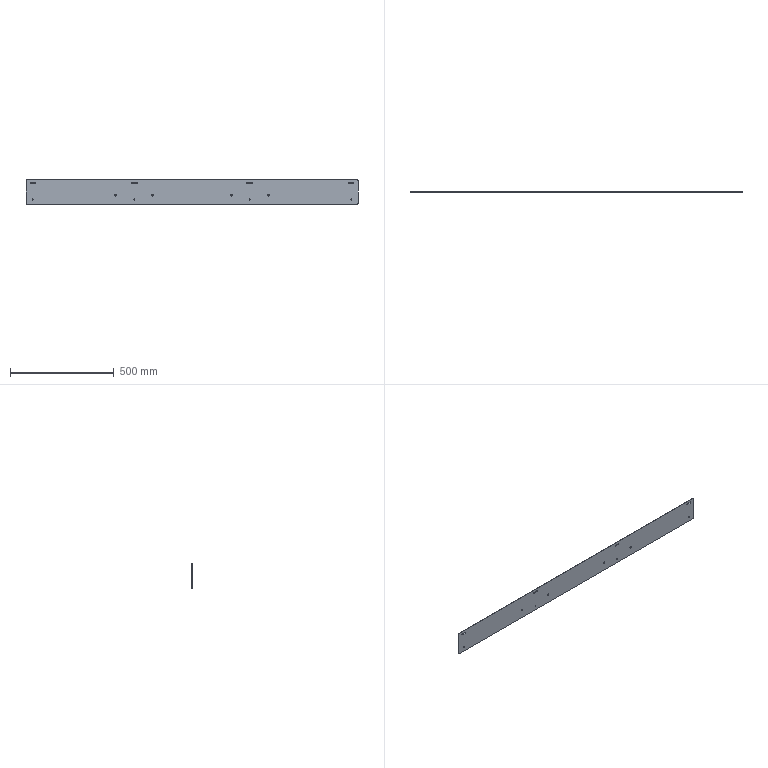Part | NX | features BREP 1 | 1 solid | 42 faces | box 1600 x 3 x 120 mm | volume 573268 mm3 | cylinder 28 | plane 14 | commonest cylinder face diameters 5.5 x8 6 x8 8 x8 10 x4
STEP:
#1=CARTESIAN_POINT('',(-800.,0.,-55.));
#2=VERTEX_POINT('',#1);
#3=CARTESIAN_POINT('',(-800.,0.,55.));
#4=VERTEX_POINT('',#3);
#5=CARTESIAN_POINT('',(-800.,0.,-55.));
#6=DIRECTION('',(0.,0.,1.));
#7=VECTOR('',#6,1000.);
#8=LINE('',#5,#7);
#9=EDGE_CURVE('',#2,#4,#8,.T.);
#10=ORIENTED_EDGE('',*,*,#9,.T.);
#11=CARTESIAN_POINT('',(-795.,0.,60.));
#12=VERTEX_POINT('',#11);
#13=CARTESIAN_POINT('',(-795.,0.,55.));
#14=DIRECTION('',(0.,1.,0.));
#15=DIRECTION('',(-1.,0.,0.));
#16=AXIS2_PLACEMENT_3D('',#13,#14,#15);
#17=CIRCLE('',#16,5.);
#18=EDGE_CURVE('',#4,#12,#17,.T.);
#19=ORIENTED_EDGE('',*,*,#18,.T.);
#20=CARTESIAN_POINT('',(795.,0.,60.));
#21=VERTEX_POINT('',#20);
#22=CARTESIAN_POINT('',(-795.,0.,60.));
#23=DIRECTION('',(1.,0.,0.));
#24=VECTOR('',#23,1000.);
#25=LINE('',#22,#24);
#26=EDGE_CURVE('',#12,#21,#25,.T.);
#27=ORIENTED_EDGE('',*,*,#26,.T.);
#28=CARTESIAN_POINT('',(800.,0.,55.));
#29=VERTEX_POINT('',#28);
#30=CARTESIAN_POINT('',(795.,0.,55.));
#31=DIRECTION('',(0.,1.,0.));
#32=DIRECTION('',(0.,0.,1.));
#33=AXIS2_PLACEMENT_3D('',#30,#31,#32);
#34=CIRCLE('',#33,5.);
#35=EDGE_CURVE('',#21,#29,#34,.T.);
#36=ORIENTED_EDGE('',*,*,#35,.T.);
#37=CARTESIAN_POINT('',(800.,0.,-55.));
#38=VERTEX_POINT('',#37);
#39=CARTESIAN_POINT('',(800.,0.,55.));
#40=DIRECTION('',(0.,0.,-1.));
#41=VECTOR('',#40,1000.);
#42=LINE('',#39,#41);
#43=EDGE_CURVE('',#29,#38,#42,.T.);
#44=ORIENTED_EDGE('',*,*,#43,.T.);
#45=CARTESIAN_POINT('',(795.,0.,-60.));
#46=VERTEX_POINT('',#45);
#47=CARTESIAN_POINT('',(795.,0.,-55.));
#48=DIRECTION('',(0.,1.,0.));
#49=DIRECTION('',(1.,0.,0.));
#50=AXIS2_PLACEMENT_3D('',#47,#48,#49);
#51=CIRCLE('',#50,5.);
#52=EDGE_CURVE('',#38,#46,#51,.T.);
#53=ORIENTED_EDGE('',*,*,#52,.T.);
#54=CARTESIAN_POINT('',(-795.,0.,-60.));
#55=VERTEX_POINT('',#54);
#56=CARTESIAN_POINT('',(795.,0.,-60.));
#57=DIRECTION('',(-1.,0.,0.));
#58=VECTOR('',#57,1000.);
#59=LINE('',#56,#58);
#60=EDGE_CURVE('',#46,#55,#59,.T.);
#61=ORIENTED_EDGE('',*,*,#60,.T.);
#62=CARTESIAN_POINT('',(-795.,0.,-55.));
#63=DIRECTION('',(0.,1.,0.));
#64=DIRECTION('',(0.,0.,-1.));
#65=AXIS2_PLACEMENT_3D('',#62,#63,#64);
#66=CIRCLE('',#65,5.);
#67=EDGE_CURVE('',#55,#2,#66,.T.);
#68=ORIENTED_EDGE('',*,*,#67,.T.);
#69=EDGE_LOOP('',(#10,#19,#27,#36,#44,#53,#61,#68));
#70=FACE_BOUND('',#69,.T.);
#71=CARTESIAN_POINT('',(-366.,0.,-15.34));
#72=VERTEX_POINT('',#71);
#73=CARTESIAN_POINT('',(-374.,0.,-15.34));
#74=VERTEX_POINT('',#73);
#75=CARTESIAN_POINT('',(-370.,0.,-15.34));
#76=DIRECTION('',(0.,1.,0.));
#77=DIRECTION('',(1.,0.,0.));
#78=AXIS2_PLACEMENT_3D('',#75,#76,#77);
#79=CIRCLE('',#78,4.);
#80=EDGE_CURVE('',#72,#74,#79,.T.);
#81=ORIENTED_EDGE('',*,*,#80,.F.);
#82=CARTESIAN_POINT('',(-370.,0.,-15.34));
#83=DIRECTION('',(0.,1.,0.));
#84=DIRECTION('',(-1.,0.,0.));
#85=AXIS2_PLACEMENT_3D('',#82,#83,#84);
#86=CIRCLE('',#85,4.);
#87=EDGE_CURVE('',#74,#72,#86,.T.);
#88=ORIENTED_EDGE('',*,*,#87,.F.);
#89=EDGE_LOOP('',(#81,#88));
#90=FACE_BOUND('',#89,.T.);
#91=CARTESIAN_POINT('',(-186.,0.,-15.34));
#92=VERTEX_POINT('',#91);
#93=CARTESIAN_POINT('',(-194.,0.,-15.34));
#94=VERTEX_POINT('',#93);
#95=CARTESIAN_POINT('',(-190.,0.,-15.34));
#96=DIRECTION('',(0.,1.,0.));
#97=DIRECTION('',(1.,0.,0.));
#98=AXIS2_PLACEMENT_3D('',#95,#96,#97);
#99=CIRCLE('',#98,4.);
#100=EDGE_CURVE('',#92,#94,#99,.T.);
#101=ORIENTED_EDGE('',*,*,#100,.F.);
#102=CARTESIAN_POINT('',(-190.,0.,-15.34));
#103=DIRECTION('',(0.,1.,0.));
#104=DIRECTION('',(-1.,0.,0.));
#105=AXIS2_PLACEMENT_3D('',#102,#103,#104);
#106=CIRCLE('',#105,4.);
#107=EDGE_CURVE('',#94,#92,#106,.T.);
#108=ORIENTED_EDGE('',*,*,#107,.F.);
#109=EDGE_LOOP('',(#101,#108));
#110=FACE_BOUND('',#109,.T.);
#111=CARTESIAN_POINT('',(194.,0.,-15.34));
#112=VERTEX_POINT('',#111);
#113=CARTESIAN_POINT('',(186.,0.,-15.34));
#114=VERTEX_POINT('',#113);
#115=CARTESIAN_POINT('',(190.,0.,-15.34));
#116=DIRECTION('',(0.,1.,0.));
#117=DIRECTION('',(1.,0.,0.));
#118=AXIS2_PLACEMENT_3D('',#115,#116,#117);
#119=CIRCLE('',#118,4.);
#120=EDGE_CURVE('',#112,#114,#119,.T.);
#121=ORIENTED_EDGE('',*,*,#120,.F.);
#122=CARTESIAN_POINT('',(190.,0.,-15.34));
#123=DIRECTION('',(0.,1.,0.));
#124=DIRECTION('',(-1.,0.,0.));
#125=AXIS2_PLACEMENT_3D('',#122,#123,#124);
#126=CIRCLE('',#125,4.);
#127=EDGE_CURVE('',#114,#112,#126,.T.);
#128=ORIENTED_EDGE('',*,*,#127,.F.);
#129=EDGE_LOOP('',(#121,#128));
#130=FACE_BOUND('',#129,.T.);
#131=CARTESIAN_POINT('',(374.,0.,-15.34));
#132=VERTEX_POINT('',#131);
#133=CARTESIAN_POINT('',(366.,0.,-15.34));
#134=VERTEX_POINT('',#133);
#135=CARTESIAN_POINT('',(370.,0.,-15.34));
#136=DIRECTION('',(0.,1.,0.));
#137=DIRECTION('',(1.,0.,0.));
#138=AXIS2_PLACEMENT_3D('',#135,#136,#137);
#139=CIRCLE('',#138,4.);
#140=EDGE_CURVE('',#132,#134,#139,.T.);
#141=ORIENTED_EDGE('',*,*,#140,.F.);
#142=CARTESIAN_POINT('',(370.,0.,-15.34));
#143=DIRECTION('',(0.,1.,0.));
#144=DIRECTION('',(-1.,0.,0.));
#145=AXIS2_PLACEMENT_3D('',#142,#143,#144);
#146=CIRCLE('',#145,4.);
#147=EDGE_CURVE('',#134,#132,#146,.T.);
#148=ORIENTED_EDGE('',*,*,#147,.F.);
#149=EDGE_LOOP('',(#141,#148));
#150=FACE_BOUND('',#149,.T.);
#151=CARTESIAN_POINT('',(757.5,0.,48.));
#152=VERTEX_POINT('',#151);
#153=CARTESIAN_POINT('',(777.5,0.,48.));
#154=VERTEX_POINT('',#153);
#155=CARTESIAN_POINT('',(757.5,0.,48.));
#156=DIRECTION('',(1.,0.,0.));
#157=VECTOR('',#156,1000.);
#158=LINE('',#155,#157);
#159=EDGE_CURVE('',#152,#154,#158,.T.);
#160=ORIENTED_EDGE('',*,*,#159,.F.);
#161=CARTESIAN_POINT('',(757.5,0.,42.));
#162=VERTEX_POINT('',#161);
#163=CARTESIAN_POINT('',(757.5,0.,45.));
#164=DIRECTION('',(0.,-1.,0.));
#165=DIRECTION('',(0.,0.,1.));
#166=AXIS2_PLACEMENT_3D('',#163,#164,#165);
#167=CIRCLE('',#166,3.);
#168=EDGE_CURVE('',#152,#162,#167,.T.);
#169=ORIENTED_EDGE('',*,*,#168,.T.);
#170=CARTESIAN_POINT('',(777.5,0.,42.));
#171=VERTEX_POINT('',#170);
#172=CARTESIAN_POINT('',(777.5,0.,42.));
#173=DIRECTION('',(-1.,0.,0.));
#174=VECTOR('',#173,1000.);
#175=LINE('',#172,#174);
#176=EDGE_CURVE('',#171,#162,#175,.T.);
#177=ORIENTED_EDGE('',*,*,#176,.F.);
#178=CARTESIAN_POINT('',(777.5,0.,45.));
#179=DIRECTION('',(0.,-1.,0.));
#180=DIRECTION('',(0.,0.,-1.));
#181=AXIS2_PLACEMENT_3D('',#178,#179,#180);
#182=CIRCLE('',#181,3.);
#183=EDGE_CURVE('',#171,#154,#182,.T.);
#184=ORIENTED_EDGE('',*,*,#183,.T.);
#185=EDGE_LOOP('',(#160,#169,#177,#184));
#186=FACE_BOUND('',#185,.T.);
#187=CARTESIAN_POINT('',(287.5,0.,42.));
#188=VERTEX_POINT('',#187);
#189=CARTESIAN_POINT('',(267.5,0.,42.));
#190=VERTEX_POINT('',#189);
#191=CARTESIAN_POINT('',(287.5,0.,42.));
#192=DIRECTION('',(-1.,0.,0.));
#193=VECTOR('',#192,1000.);
#194=LINE('',#191,#193);
#195=EDGE_CURVE('',#188,#190,#194,.T.);
#196=ORIENTED_EDGE('',*,*,#195,.F.);
#197=CARTESIAN_POINT('',(287.5,0.,48.));
#198=VERTEX_POINT('',#197);
#199=CARTESIAN_POINT('',(287.5,0.,45.));
#200=DIRECTION('',(0.,-1.,0.));
#201=DIRECTION('',(0.,0.,-1.));
#202=AXIS2_PLACEMENT_3D('',#199,#200,#201);
#203=CIRCLE('',#202,3.);
#204=EDGE_CURVE('',#188,#198,#203,.T.);
#205=ORIENTED_EDGE('',*,*,#204,.T.);
#206=CARTESIAN_POINT('',(267.5,0.,48.));
#207=VERTEX_POINT('',#206);
#208=CARTESIAN_POINT('',(267.5,0.,48.));
#209=DIRECTION('',(1.,0.,0.));
#210=VECTOR('',#209,1000.);
#211=LINE('',#208,#210);
#212=EDGE_CURVE('',#207,#198,#211,.T.);
#213=ORIENTED_EDGE('',*,*,#212,.F.);
#214=CARTESIAN_POINT('',(267.5,0.,45.));
#215=DIRECTION('',(0.,-1.,0.));
#216=DIRECTION('',(0.,0.,1.));
#217=AXIS2_PLACEMENT_3D('',#214,#215,#216);
#218=CIRCLE('',#217,3.);
#219=EDGE_CURVE('',#207,#190,#218,.T.);
#220=ORIENTED_EDGE('',*,*,#219,.T.);
#221=EDGE_LOOP('',(#196,#205,#213,#220));
#222=FACE_BOUND('',#221,.T.);
#223=CARTESIAN_POINT('',(-777.5,0.,48.));
#224=VERTEX_POINT('',#223);
#225=CARTESIAN_POINT('',(-777.5,0.,42.));
#226=VERTEX_POINT('',#225);
#227=CARTESIAN_POINT('',(-777.5,0.,45.));
#228=DIRECTION('',(0.,-1.,0.));
#229=DIRECTION('',(0.,0.,1.));
#230=AXIS2_PLACEMENT_3D('',#227,#228,#229);
#231=CIRCLE('',#230,3.);
#232=EDGE_CURVE('',#224,#226,#231,.T.);
#233=ORIENTED_EDGE('',*,*,#232,.T.);
#234=CARTESIAN_POINT('',(-757.5,0.,42.));
#235=VERTEX_POINT('',#234);
#236=CARTESIAN_POINT('',(-757.5,0.,42.));
#237=DIRECTION('',(-1.,0.,0.));
#238=VECTOR('',#237,1000.);
#239=LINE('',#236,#238);
#240=EDGE_CURVE('',#235,#226,#239,.T.);
#241=ORIENTED_EDGE('',*,*,#240,.F.);
#242=CARTESIAN_POINT('',(-757.5,0.,48.));
#243=VERTEX_POINT('',#242);
#244=CARTESIAN_POINT('',(-757.5,0.,45.));
#245=DIRECTION('',(0.,-1.,0.));
#246=DIRECTION('',(0.,0.,-1.));
#247=AXIS2_PLACEMENT_3D('',#244,#245,#246);
#248=CIRCLE('',#247,3.);
#249=EDGE_CURVE('',#235,#243,#248,.T.);
#250=ORIENTED_EDGE('',*,*,#249,.T.);
#251=CARTESIAN_POINT('',(-777.5,0.,48.));
#252=DIRECTION('',(1.,0.,0.));
#253=VECTOR('',#252,1000.);
#254=LINE('',#251,#253);
#255=EDGE_CURVE('',#224,#243,#254,.T.);
#256=ORIENTED_EDGE('',*,*,#255,.F.);
#257=EDGE_LOOP('',(#233,#241,#250,#256));
#258=FACE_BOUND('',#257,.T.);
#259=CARTESIAN_POINT('',(-267.5,0.,42.));
#260=VERTEX_POINT('',#259);
#261=CARTESIAN_POINT('',(-267.5,0.,48.));
#262=VERTEX_POINT('',#261);
#263=CARTESIAN_POINT('',(-267.5,0.,45.));
#264=DIRECTION('',(0.,-1.,0.));
#265=DIRECTION('',(0.,0.,-1.));
#266=AXIS2_PLACEMENT_3D('',#263,#264,#265);
#267=CIRCLE('',#266,3.);
#268=EDGE_CURVE('',#260,#262,#267,.T.);
#269=ORIENTED_EDGE('',*,*,#268,.T.);
#270=CARTESIAN_POINT('',(-287.5,0.,48.));
#271=VERTEX_POINT('',#270);
#272=CARTESIAN_POINT('',(-287.5,0.,48.));
#273=DIRECTION('',(1.,0.,0.));
#274=VECTOR('',#273,1000.);
#275=LINE('',#272,#274);
#276=EDGE_CURVE('',#271,#262,#275,.T.);
#277=ORIENTED_EDGE('',*,*,#276,.F.);
#278=CARTESIAN_POINT('',(-287.5,0.,42.));
#279=VERTEX_POINT('',#278);
#280=CARTESIAN_POINT('',(-287.5,0.,45.));
#281=DIRECTION('',(0.,-1.,0.));
#282=DIRECTION('',(0.,0.,1.));
#283=AXIS2_PLACEMENT_3D('',#280,#281,#282);
#284=CIRCLE('',#283,3.);
#285=EDGE_CURVE('',#271,#279,#284,.T.);
#286=ORIENTED_EDGE('',*,*,#285,.T.);
#287=CARTESIAN_POINT('',(-267.5,0.,42.));
#288=DIRECTION('',(-1.,0.,0.));
#289=VECTOR('',#288,1000.);
#290=LINE('',#287,#289);
#291=EDGE_CURVE('',#260,#279,#290,.T.);
#292=ORIENTED_EDGE('',*,*,#291,.F.);
#293=EDGE_LOOP('',(#269,#277,#286,#292));
#294=FACE_BOUND('',#293,.T.);
#295=CARTESIAN_POINT('',(770.25,0.,-36.));
#296=VERTEX_POINT('',#295);
#297=CARTESIAN_POINT('',(764.75,0.,-36.));
#298=VERTEX_POINT('',#297);
#299=CARTESIAN_POINT('',(767.5,0.,-36.));
#300=DIRECTION('',(0.,1.,0.));
#301=DIRECTION('',(1.,0.,0.));
#302=AXIS2_PLACEMENT_3D('',#299,#300,#301);
#303=CIRCLE('',#302,2.75);
#304=EDGE_CURVE('',#296,#298,#303,.T.);
#305=ORIENTED_EDGE('',*,*,#304,.F.);
#306=CARTESIAN_POINT('',(767.5,0.,-36.));
#307=DIRECTION('',(0.,1.,0.));
#308=DIRECTION('',(-1.,0.,0.));
#309=AXIS2_PLACEMENT_3D('',#306,#307,#308);
#310=CIRCLE('',#309,2.75);
#311=EDGE_CURVE('',#298,#296,#310,.T.);
#312=ORIENTED_EDGE('',*,*,#311,.F.);
#313=EDGE_LOOP('',(#305,#312));
#314=FACE_BOUND('',#313,.T.);
#315=CARTESIAN_POINT('',(-764.75,0.,-36.));
#316=VERTEX_POINT('',#315);
#317=CARTESIAN_POINT('',(-770.25,0.,-36.));
#318=VERTEX_POINT('',#317);
#319=CARTESIAN_POINT('',(-767.5,0.,-36.));
#320=DIRECTION('',(0.,1.,0.));
#321=DIRECTION('',(1.,0.,0.));
#322=AXIS2_PLACEMENT_3D('',#319,#320,#321);
#323=CIRCLE('',#322,2.75);
#324=EDGE_CURVE('',#316,#318,#323,.T.);
#325=ORIENTED_EDGE('',*,*,#324,.F.);
#326=CARTESIAN_POINT('',(-767.5,0.,-36.));
#327=DIRECTION('',(0.,1.,0.));
#328=DIRECTION('',(-1.,0.,0.));
#329=AXIS2_PLACEMENT_3D('',#326,#327,#328);
#330=CIRCLE('',#329,2.75);
#331=EDGE_CURVE('',#318,#316,#330,.T.);
#332=ORIENTED_EDGE('',*,*,#331,.F.);
#333=EDGE_LOOP('',(#325,#332));
#334=FACE_BOUND('',#333,.T.);
#335=CARTESIAN_POINT('',(-274.75,0.,-36.));
#336=VERTEX_POINT('',#335);
#337=CARTESIAN_POINT('',(-280.25,0.,-36.));
#338=VERTEX_POINT('',#337);
#339=CARTESIAN_POINT('',(-277.5,0.,-36.));
#340=DIRECTION('',(0.,1.,0.));
#341=DIRECTION('',(1.,0.,0.));
#342=AXIS2_PLACEMENT_3D('',#339,#340,#341);
#343=CIRCLE('',#342,2.75);
#344=EDGE_CURVE('',#336,#338,#343,.T.);
#345=ORIENTED_EDGE('',*,*,#344,.F.);
#346=CARTESIAN_POINT('',(-277.5,0.,-36.));
#347=DIRECTION('',(0.,1.,0.));
#348=DIRECTION('',(-1.,0.,0.));
#349=AXIS2_PLACEMENT_3D('',#346,#347,#348);
#350=CIRCLE('',#349,2.75);
#351=EDGE_CURVE('',#338,#336,#350,.T.);
#352=ORIENTED_EDGE('',*,*,#351,.F.);
#353=EDGE_LOOP('',(#345,#352));
#354=FACE_BOUND('',#353,.T.);
#355=CARTESIAN_POINT('',(280.25,0.,-36.));
#356=VERTEX_POINT('',#355);
#357=CARTESIAN_POINT('',(274.75,0.,-36.));
#358=VERTEX_POINT('',#357);
#359=CARTESIAN_POINT('',(277.5,0.,-36.));
#360=DIRECTION('',(0.,1.,0.));
#361=DIRECTION('',(1.,0.,0.));
#362=AXIS2_PLACEMENT_3D('',#359,#360,#361);
#363=CIRCLE('',#362,2.75);
#364=EDGE_CURVE('',#356,#358,#363,.T.);
#365=ORIENTED_EDGE('',*,*,#364,.F.);
#366=CARTESIAN_POINT('',(277.5,0.,-36.));
#367=DIRECTION('',(0.,1.,0.));
#368=DIRECTION('',(-1.,0.,0.));
#369=AXIS2_PLACEMENT_3D('',#366,#367,#368);
#370=CIRCLE('',#369,2.75);
#371=EDGE_CURVE('',#358,#356,#370,.T.);
#372=ORIENTED_EDGE('',*,*,#371,.F.);
#373=EDGE_LOOP('',(#365,#372));
#374=FACE_BOUND('',#373,.T.);
#375=CARTESIAN_POINT('',(0.,0.,0.));
#376=DIRECTION('',(0.,1.,0.));
#377=DIRECTION('',(1.,0.,0.));
#378=AXIS2_PLACEMENT_3D('',#375,#376,#377);
#379=PLANE('',#378);
#380=ADVANCED_FACE('',(#70,#90,#110,#130,#150,#186,#222,#258,#294,#314,#334,#354,#374),#379,.T.);
#381=CARTESIAN_POINT('',(-795.,-3.,-60.));
#382=VERTEX_POINT('',#381);
#383=CARTESIAN_POINT('',(-795.,-3.,-60.));
#384=DIRECTION('',(0.,1.,0.));
#385=VECTOR('',#384,1000.);
#386=LINE('',#383,#385);
#387=EDGE_CURVE('',#382,#55,#386,.T.);
#388=ORIENTED_EDGE('',*,*,#387,.F.);
#389=CARTESIAN_POINT('',(-800.,-3.,-55.));
#390=VERTEX_POINT('',#389);
#391=CARTESIAN_POINT('',(-795.,-3.,-55.));
#392=DIRECTION('',(0.,-1.,0.));
#393=DIRECTION('',(-1.,0.,0.));
#394=AXIS2_PLACEMENT_3D('',#391,#392,#393);
#395=CIRCLE('',#394,5.);
#396=EDGE_CURVE('',#390,#382,#395,.T.);
#397=ORIENTED_EDGE('',*,*,#396,.F.);
#398=CARTESIAN_POINT('',(-800.,-3.,-55.));
#399=DIRECTION('',(0.,1.,0.));
#400=VECTOR('',#399,1000.);
#401=LINE('',#398,#400);
#402=EDGE_CURVE('',#390,#2,#401,.T.);
#403=ORIENTED_EDGE('',*,*,#402,.T.);
#404=ORIENTED_EDGE('',*,*,#67,.F.);
#405=EDGE_LOOP('',(#388,#397,#403,#404));
#406=FACE_BOUND('',#405,.T.);
#407=CARTESIAN_POINT('',(-795.,-9.316,-55.));
#408=DIRECTION('',(0.,1.,0.));
#409=DIRECTION('',(0.,0.,-1.));
#410=AXIS2_PLACEMENT_3D('',#407,#408,#409);
#411=CYLINDRICAL_SURFACE('',#410,5.);
#412=ADVANCED_FACE('',(#406),#411,.T.);
#413=CARTESIAN_POINT('',(-800.,-3.,55.));
#414=VERTEX_POINT('',#413);
#415=CARTESIAN_POINT('',(-800.,-3.,-55.));
#416=DIRECTION('',(0.,0.,1.));
#417=VECTOR('',#416,1000.);
#418=LINE('',#415,#417);
#419=EDGE_CURVE('',#390,#414,#418,.T.);
#420=ORIENTED_EDGE('',*,*,#419,.T.);
#421=CARTESIAN_POINT('',(-800.,-3.,55.));
#422=DIRECTION('',(0.,1.,0.));
#423=VECTOR('',#422,1000.);
#424=LINE('',#421,#423);
#425=EDGE_CURVE('',#414,#4,#424,.T.);
#426=ORIENTED_EDGE('',*,*,#425,.T.);
#427=ORIENTED_EDGE('',*,*,#9,.F.);
#428=ORIENTED_EDGE('',*,*,#402,.F.);
#429=EDGE_LOOP('',(#420,#426,#427,#428));
#430=FACE_BOUND('',#429,.T.);
#431=CARTESIAN_POINT('',(-800.,-1.5,0.));
#432=DIRECTION('',(-1.,0.,0.));
#433=DIRECTION('',(0.,0.,1.));
#434=AXIS2_PLACEMENT_3D('',#431,#432,#433);
#435=PLANE('',#434);
#436=ADVANCED_FACE('',(#430),#435,.T.);
#437=ORIENTED_EDGE('',*,*,#425,.F.);
#438=CARTESIAN_POINT('',(-795.,-3.,60.));
#439=VERTEX_POINT('',#438);
#440=CARTESIAN_POINT('',(-795.,-3.,55.));
#441=DIRECTION('',(0.,-1.,0.));
#442=DIRECTION('',(0.,0.,1.));
#443=AXIS2_PLACEMENT_3D('',#440,#441,#442);
#444=CIRCLE('',#443,5.);
#445=EDGE_CURVE('',#439,#414,#444,.T.);
#446=ORIENTED_EDGE('',*,*,#445,.F.);
#447=CARTESIAN_POINT('',(-795.,-3.,60.));
#448=DIRECTION('',(0.,1.,0.));
#449=VECTOR('',#448,1000.);
#450=LINE('',#447,#449);
#451=EDGE_CURVE('',#439,#12,#450,.T.);
#452=ORIENTED_EDGE('',*,*,#451,.T.);
#453=ORIENTED_EDGE('',*,*,#18,.F.);
#454=EDGE_LOOP('',(#437,#446,#452,#453));
#455=FACE_BOUND('',#454,.T.);
#456=CARTESIAN_POINT('',(-795.,-9.316,55.));
#457=DIRECTION('',(0.,1.,0.));
#458=DIRECTION('',(-1.,0.,0.));
#459=AXIS2_PLACEMENT_3D('',#456,#457,#458);
#460=CYLINDRICAL_SURFACE('',#459,5.);
#461=ADVANCED_FACE('',(#455),#460,.T.);
#462=CARTESIAN_POINT('',(795.,-3.,60.));
#463=VERTEX_POINT('',#462);
#464=CARTESIAN_POINT('',(-795.,-3.,60.));
#465=DIRECTION('',(1.,0.,0.));
#466=VECTOR('',#465,1000.);
#467=LINE('',#464,#466);
#468=EDGE_CURVE('',#439,#463,#467,.T.);
#469=ORIENTED_EDGE('',*,*,#468,.T.);
#470=CARTESIAN_POINT('',(795.,-3.,60.));
#471=DIRECTION('',(0.,1.,0.));
#472=VECTOR('',#471,1000.);
#473=LINE('',#470,#472);
#474=EDGE_CURVE('',#463,#21,#473,.T.);
#475=ORIENTED_EDGE('',*,*,#474,.T.);
#476=ORIENTED_EDGE('',*,*,#26,.F.);
#477=ORIENTED_EDGE('',*,*,#451,.F.);
#478=EDGE_LOOP('',(#469,#475,#476,#477));
#479=FACE_BOUND('',#478,.T.);
#480=CARTESIAN_POINT('',(0.,-1.5,60.));
#481=DIRECTION('',(0.,0.,1.));
#482=DIRECTION('',(1.,0.,0.));
#483=AXIS2_PLACEMENT_3D('',#480,#481,#482);
#484=PLANE('',#483);
#485=ADVANCED_FACE('',(#479),#484,.T.);
#486=ORIENTED_EDGE('',*,*,#474,.F.);
#487=CARTESIAN_POINT('',(800.,-3.,55.));
#488=VERTEX_POINT('',#487);
#489=CARTESIAN_POINT('',(795.,-3.,55.));
#490=DIRECTION('',(0.,-1.,0.));
#491=DIRECTION('',(1.,0.,0.));
#492=AXIS2_PLACEMENT_3D('',#489,#490,#491);
#493=CIRCLE('',#492,5.);
#494=EDGE_CURVE('',#488,#463,#493,.T.);
#495=ORIENTED_EDGE('',*,*,#494,.F.);
#496=CARTESIAN_POINT('',(800.,-3.,55.));
#497=DIRECTION('',(0.,1.,0.));
#498=VECTOR('',#497,1000.);
#499=LINE('',#496,#498);
#500=EDGE_CURVE('',#488,#29,#499,.T.);
#501=ORIENTED_EDGE('',*,*,#500,.T.);
#502=ORIENTED_EDGE('',*,*,#35,.F.);
#503=EDGE_LOOP('',(#486,#495,#501,#502));
#504=FACE_BOUND('',#503,.T.);
#505=CARTESIAN_POINT('',(795.,-9.316,55.));
#506=DIRECTION('',(0.,1.,0.));
#507=DIRECTION('',(0.,0.,1.));
#508=AXIS2_PLACEMENT_3D('',#505,#506,#507);
#509=CYLINDRICAL_SURFACE('',#508,5.);
#510=ADVANCED_FACE('',(#504),#509,.T.);
#511=ORIENTED_EDGE('',*,*,#43,.F.);
#512=ORIENTED_EDGE('',*,*,#500,.F.);
#513=CARTESIAN_POINT('',(800.,-3.,-55.));
#514=VERTEX_POINT('',#513);
#515=CARTESIAN_POINT('',(800.,-3.,55.));
#516=DIRECTION('',(0.,0.,-1.));
#517=VECTOR('',#516,1000.);
#518=LINE('',#515,#517);
#519=EDGE_CURVE('',#488,#514,#518,.T.);
#520=ORIENTED_EDGE('',*,*,#519,.T.);
#521=CARTESIAN_POINT('',(800.,-3.,-55.));
#522=DIRECTION('',(0.,1.,0.));
#523=VECTOR('',#522,1000.);
#524=LINE('',#521,#523);
#525=EDGE_CURVE('',#514,#38,#524,.T.);
#526=ORIENTED_EDGE('',*,*,#525,.T.);
#527=EDGE_LOOP('',(#511,#512,#520,#526));
#528=FACE_BOUND('',#527,.T.);
#529=CARTESIAN_POINT('',(800.,-1.5,0.));
#530=DIRECTION('',(1.,0.,0.));
#531=DIRECTION('',(0.,1.,0.));
#532=AXIS2_PLACEMENT_3D('',#529,#530,#531);
#533=PLANE('',#532);
#534=ADVANCED_FACE('',(#528),#533,.T.);
#535=ORIENTED_EDGE('',*,*,#525,.F.);
#536=CARTESIAN_POINT('',(795.,-3.,-60.));
#537=VERTEX_POINT('',#536);
#538=CARTESIAN_POINT('',(795.,-3.,-55.));
#539=DIRECTION('',(0.,-1.,0.));
#540=DIRECTION('',(0.,0.,-1.));
#541=AXIS2_PLACEMENT_3D('',#538,#539,#540);
#542=CIRCLE('',#541,5.);
#543=EDGE_CURVE('',#537,#514,#542,.T.);
#544=ORIENTED_EDGE('',*,*,#543,.F.);
#545=CARTESIAN_POINT('',(795.,-3.,-60.));
#546=DIRECTION('',(0.,1.,0.));
#547=VECTOR('',#546,1000.);
#548=LINE('',#545,#547);
#549=EDGE_CURVE('',#537,#46,#548,.T.);
#550=ORIENTED_EDGE('',*,*,#549,.T.);
#551=ORIENTED_EDGE('',*,*,#52,.F.);
#552=EDGE_LOOP('',(#535,#544,#550,#551));
#553=FACE_BOUND('',#552,.T.);
#554=CARTESIAN_POINT('',(795.,-9.316,-55.));
#555=DIRECTION('',(0.,1.,0.));
#556=DIRECTION('',(1.,0.,0.));
#557=AXIS2_PLACEMENT_3D('',#554,#555,#556);
#558=CYLINDRICAL_SURFACE('',#557,5.);
#559=ADVANCED_FACE('',(#553),#558,.T.);
#560=ORIENTED_EDGE('',*,*,#60,.F.);
#561=ORIENTED_EDGE('',*,*,#549,.F.);
#562=CARTESIAN_POINT('',(795.,-3.,-60.));
#563=DIRECTION('',(-1.,0.,0.));
#564=VECTOR('',#563,1000.);
#565=LINE('',#562,#564);
#566=EDGE_CURVE('',#537,#382,#565,.T.);
#567=ORIENTED_EDGE('',*,*,#566,.T.);
#568=ORIENTED_EDGE('',*,*,#387,.T.);
#569=EDGE_LOOP('',(#560,#561,#567,#568));
#570=FACE_BOUND('',#569,.T.);
#571=CARTESIAN_POINT('',(0.,-1.5,-60.));
#572=DIRECTION('',(0.,0.,-1.));
#573=DIRECTION('',(0.,-1.,0.));
#574=AXIS2_PLACEMENT_3D('',#571,#572,#573);
#575=PLANE('',#574);
#576=ADVANCED_FACE('',(#570),#575,.T.);
#577=ORIENTED_EDGE('',*,*,#566,.F.);
#578=ORIENTED_EDGE('',*,*,#543,.T.);
#579=ORIENTED_EDGE('',*,*,#519,.F.);
#580=ORIENTED_EDGE('',*,*,#494,.T.);
#581=ORIENTED_EDGE('',*,*,#468,.F.);
#582=ORIENTED_EDGE('',*,*,#445,.T.);
#583=ORIENTED_EDGE('',*,*,#419,.F.);
#584=ORIENTED_EDGE('',*,*,#396,.T.);
#585=EDGE_LOOP('',(#577,#578,#579,#580,#581,#582,#583,#584));
#586=FACE_BOUND('',#585,.T.);
#587=CARTESIAN_POINT('',(374.,-3.,-15.34));
#588=VERTEX_POINT('',#587);
#589=CARTESIAN_POINT('',(366.,-3.,-15.34));
#590=VERTEX_POINT('',#589);
#591=CARTESIAN_POINT('',(370.,-3.,-15.34));
#592=DIRECTION('',(0.,1.,0.));
#593=DIRECTION('',(1.,0.,0.));
#594=AXIS2_PLACEMENT_3D('',#591,#592,#593);
#595=CIRCLE('',#594,4.);
#596=EDGE_CURVE('',#588,#590,#595,.T.);
#597=ORIENTED_EDGE('',*,*,#596,.T.);
#598=CARTESIAN_POINT('',(370.,-3.,-15.34));
#599=DIRECTION('',(0.,1.,0.));
#600=DIRECTION('',(-1.,0.,0.));
#601=AXIS2_PLACEMENT_3D('',#598,#599,#600);
#602=CIRCLE('',#601,4.);
#603=EDGE_CURVE('',#590,#588,#602,.T.);
#604=ORIENTED_EDGE('',*,*,#603,.T.);
#605=EDGE_LOOP('',(#597,#604));
#606=FACE_BOUND('',#605,.T.);
#607=CARTESIAN_POINT('',(194.,-3.,-15.34));
#608=VERTEX_POINT('',#607);
#609=CARTESIAN_POINT('',(186.,-3.,-15.34));
#610=VERTEX_POINT('',#609);
#611=CARTESIAN_POINT('',(190.,-3.,-15.34));
#612=DIRECTION('',(0.,1.,0.));
#613=DIRECTION('',(1.,0.,0.));
#614=AXIS2_PLACEMENT_3D('',#611,#612,#613);
#615=CIRCLE('',#614,4.);
#616=EDGE_CURVE('',#608,#610,#615,.T.);
#617=ORIENTED_EDGE('',*,*,#616,.T.);
#618=CARTESIAN_POINT('',(190.,-3.,-15.34));
#619=DIRECTION('',(0.,1.,0.));
#620=DIRECTION('',(-1.,0.,0.));
#621=AXIS2_PLACEMENT_3D('',#618,#619,#620);
#622=CIRCLE('',#621,4.);
#623=EDGE_CURVE('',#610,#608,#622,.T.);
#624=ORIENTED_EDGE('',*,*,#623,.T.);
#625=EDGE_LOOP('',(#617,#624));
#626=FACE_BOUND('',#625,.T.);
#627=CARTESIAN_POINT('',(-186.,-3.,-15.34));
#628=VERTEX_POINT('',#627);
#629=CARTESIAN_POINT('',(-194.,-3.,-15.34));
#630=VERTEX_POINT('',#629);
#631=CARTESIAN_POINT('',(-190.,-3.,-15.34));
#632=DIRECTION('',(0.,1.,0.));
#633=DIRECTION('',(1.,0.,0.));
#634=AXIS2_PLACEMENT_3D('',#631,#632,#633);
#635=CIRCLE('',#634,4.);
#636=EDGE_CURVE('',#628,#630,#635,.T.);
#637=ORIENTED_EDGE('',*,*,#636,.T.);
#638=CARTESIAN_POINT('',(-190.,-3.,-15.34));
#639=DIRECTION('',(0.,1.,0.));
#640=DIRECTION('',(-1.,0.,0.));
#641=AXIS2_PLACEMENT_3D('',#638,#639,#640);
#642=CIRCLE('',#641,4.);
#643=EDGE_CURVE('',#630,#628,#642,.T.);
#644=ORIENTED_EDGE('',*,*,#643,.T.);
#645=EDGE_LOOP('',(#637,#644));
#646=FACE_BOUND('',#645,.T.);
#647=CARTESIAN_POINT('',(-366.,-3.,-15.34));
#648=VERTEX_POINT('',#647);
#649=CARTESIAN_POINT('',(-374.,-3.,-15.34));
#650=VERTEX_POINT('',#649);
#651=CARTESIAN_POINT('',(-370.,-3.,-15.34));
#652=DIRECTION('',(0.,1.,0.));
#653=DIRECTION('',(1.,0.,0.));
#654=AXIS2_PLACEMENT_3D('',#651,#652,#653);
#655=CIRCLE('',#654,4.);
#656=EDGE_CURVE('',#648,#650,#655,.T.);
#657=ORIENTED_EDGE('',*,*,#656,.T.);
#658=CARTESIAN_POINT('',(-370.,-3.,-15.34));
#659=DIRECTION('',(0.,1.,0.));
#660=DIRECTION('',(-1.,0.,0.));
#661=AXIS2_PLACEMENT_3D('',#658,#659,#660);
#662=CIRCLE('',#661,4.);
#663=EDGE_CURVE('',#650,#648,#662,.T.);
#664=ORIENTED_EDGE('',*,*,#663,.T.);
#665=EDGE_LOOP('',(#657,#664));
#666=FACE_BOUND('',#665,.T.);
#667=CARTESIAN_POINT('',(-287.5,-3.,48.));
#668=VERTEX_POINT('',#667);
#669=CARTESIAN_POINT('',(-287.5,-3.,42.));
#670=VERTEX_POINT('',#669);
#671=CARTESIAN_POINT('',(-287.5,-3.,45.));
#672=DIRECTION('',(0.,-1.,0.));
#673=DIRECTION('',(0.,0.,1.));
#674=AXIS2_PLACEMENT_3D('',#671,#672,#673);
#675=CIRCLE('',#674,3.);
#676=EDGE_CURVE('',#668,#670,#675,.T.);
#677=ORIENTED_EDGE('',*,*,#676,.F.);
#678=CARTESIAN_POINT('',(-267.5,-3.,48.));
#679=VERTEX_POINT('',#678);
#680=CARTESIAN_POINT('',(-287.5,-3.,48.));
#681=DIRECTION('',(1.,0.,0.));
#682=VECTOR('',#681,1000.);
#683=LINE('',#680,#682);
#684=EDGE_CURVE('',#668,#679,#683,.T.);
#685=ORIENTED_EDGE('',*,*,#684,.T.);
#686=CARTESIAN_POINT('',(-267.5,-3.,42.));
#687=VERTEX_POINT('',#686);
#688=CARTESIAN_POINT('',(-267.5,-3.,45.));
#689=DIRECTION('',(0.,-1.,0.));
#690=DIRECTION('',(0.,0.,-1.));
#691=AXIS2_PLACEMENT_3D('',#688,#689,#690);
#692=CIRCLE('',#691,3.);
#693=EDGE_CURVE('',#687,#679,#692,.T.);
#694=ORIENTED_EDGE('',*,*,#693,.F.);
#695=CARTESIAN_POINT('',(-267.5,-3.,42.));
#696=DIRECTION('',(-1.,0.,0.));
#697=VECTOR('',#696,1000.);
#698=LINE('',#695,#697);
#699=EDGE_CURVE('',#687,#670,#698,.T.);
#700=ORIENTED_EDGE('',*,*,#699,.T.);
#701=EDGE_LOOP('',(#677,#685,#694,#700));
#702=FACE_BOUND('',#701,.T.);
#703=CARTESIAN_POINT('',(-757.5,-3.,42.));
#704=VERTEX_POINT('',#703);
#705=CARTESIAN_POINT('',(-757.5,-3.,48.));
#706=VERTEX_POINT('',#705);
#707=CARTESIAN_POINT('',(-757.5,-3.,45.));
#708=DIRECTION('',(0.,-1.,0.));
#709=DIRECTION('',(0.,0.,-1.));
#710=AXIS2_PLACEMENT_3D('',#707,#708,#709);
#711=CIRCLE('',#710,3.);
#712=EDGE_CURVE('',#704,#706,#711,.T.);
#713=ORIENTED_EDGE('',*,*,#712,.F.);
#714=CARTESIAN_POINT('',(-777.5,-3.,42.));
#715=VERTEX_POINT('',#714);
#716=CARTESIAN_POINT('',(-757.5,-3.,42.));
#717=DIRECTION('',(-1.,0.,0.));
#718=VECTOR('',#717,1000.);
#719=LINE('',#716,#718);
#720=EDGE_CURVE('',#704,#715,#719,.T.);
#721=ORIENTED_EDGE('',*,*,#720,.T.);
#722=CARTESIAN_POINT('',(-777.5,-3.,48.));
#723=VERTEX_POINT('',#722);
#724=CARTESIAN_POINT('',(-777.5,-3.,45.));
#725=DIRECTION('',(0.,-1.,0.));
#726=DIRECTION('',(0.,0.,1.));
#727=AXIS2_PLACEMENT_3D('',#724,#725,#726);
#728=CIRCLE('',#727,3.);
#729=EDGE_CURVE('',#723,#715,#728,.T.);
#730=ORIENTED_EDGE('',*,*,#729,.F.);
#731=CARTESIAN_POINT('',(-777.5,-3.,48.));
#732=DIRECTION('',(1.,0.,0.));
#733=VECTOR('',#732,1000.);
#734=LINE('',#731,#733);
#735=EDGE_CURVE('',#723,#706,#734,.T.);
#736=ORIENTED_EDGE('',*,*,#735,.T.);
#737=EDGE_LOOP('',(#713,#721,#730,#736));
#738=FACE_BOUND('',#737,.T.);
#739=CARTESIAN_POINT('',(267.5,-3.,48.));
#740=VERTEX_POINT('',#739);
#741=CARTESIAN_POINT('',(287.5,-3.,48.));
#742=VERTEX_POINT('',#741);
#743=CARTESIAN_POINT('',(267.5,-3.,48.));
#744=DIRECTION('',(1.,0.,0.));
#745=VECTOR('',#744,1000.);
#746=LINE('',#743,#745);
#747=EDGE_CURVE('',#740,#742,#746,.T.);
#748=ORIENTED_EDGE('',*,*,#747,.T.);
#749=CARTESIAN_POINT('',(287.5,-3.,42.));
#750=VERTEX_POINT('',#749);
#751=CARTESIAN_POINT('',(287.5,-3.,45.));
#752=DIRECTION('',(0.,-1.,0.));
#753=DIRECTION('',(0.,0.,-1.));
#754=AXIS2_PLACEMENT_3D('',#751,#752,#753);
#755=CIRCLE('',#754,3.);
#756=EDGE_CURVE('',#750,#742,#755,.T.);
#757=ORIENTED_EDGE('',*,*,#756,.F.);
#758=CARTESIAN_POINT('',(267.5,-3.,42.));
#759=VERTEX_POINT('',#758);
#760=CARTESIAN_POINT('',(287.5,-3.,42.));
#761=DIRECTION('',(-1.,0.,0.));
#762=VECTOR('',#761,1000.);
#763=LINE('',#760,#762);
#764=EDGE_CURVE('',#750,#759,#763,.T.);
#765=ORIENTED_EDGE('',*,*,#764,.T.);
#766=CARTESIAN_POINT('',(267.5,-3.,45.));
#767=DIRECTION('',(0.,-1.,0.));
#768=DIRECTION('',(0.,0.,1.));
#769=AXIS2_PLACEMENT_3D('',#766,#767,#768);
#770=CIRCLE('',#769,3.);
#771=EDGE_CURVE('',#740,#759,#770,.T.);
#772=ORIENTED_EDGE('',*,*,#771,.F.);
#773=EDGE_LOOP('',(#748,#757,#765,#772));
#774=FACE_BOUND('',#773,.T.);
#775=CARTESIAN_POINT('',(777.5,-3.,42.));
#776=VERTEX_POINT('',#775);
#777=CARTESIAN_POINT('',(757.5,-3.,42.));
#778=VERTEX_POINT('',#777);
#779=CARTESIAN_POINT('',(777.5,-3.,42.));
#780=DIRECTION('',(-1.,0.,0.));
#781=VECTOR('',#780,1000.);
#782=LINE('',#779,#781);
#783=EDGE_CURVE('',#776,#778,#782,.T.);
#784=ORIENTED_EDGE('',*,*,#783,.T.);
#785=CARTESIAN_POINT('',(757.5,-3.,48.));
#786=VERTEX_POINT('',#785);
#787=CARTESIAN_POINT('',(757.5,-3.,45.));
#788=DIRECTION('',(0.,-1.,0.));
#789=DIRECTION('',(0.,0.,1.));
#790=AXIS2_PLACEMENT_3D('',#787,#788,#789);
#791=CIRCLE('',#790,3.);
#792=EDGE_CURVE('',#786,#778,#791,.T.);
#793=ORIENTED_EDGE('',*,*,#792,.F.);
#794=CARTESIAN_POINT('',(777.5,-3.,48.));
#795=VERTEX_POINT('',#794);
#796=CARTESIAN_POINT('',(757.5,-3.,48.));
#797=DIRECTION('',(1.,0.,0.));
#798=VECTOR('',#797,1000.);
#799=LINE('',#796,#798);
#800=EDGE_CURVE('',#786,#795,#799,.T.);
#801=ORIENTED_EDGE('',*,*,#800,.T.);
#802=CARTESIAN_POINT('',(777.5,-3.,45.));
#803=DIRECTION('',(0.,-1.,0.));
#804=DIRECTION('',(0.,0.,-1.));
#805=AXIS2_PLACEMENT_3D('',#802,#803,#804);
#806=CIRCLE('',#805,3.);
#807=EDGE_CURVE('',#776,#795,#806,.T.);
#808=ORIENTED_EDGE('',*,*,#807,.F.);
#809=EDGE_LOOP('',(#784,#793,#801,#808));
#810=FACE_BOUND('',#809,.T.);
#811=CARTESIAN_POINT('',(770.25,-3.,-36.));
#812=VERTEX_POINT('',#811);
#813=CARTESIAN_POINT('',(764.75,-3.,-36.));
#814=VERTEX_POINT('',#813);
#815=CARTESIAN_POINT('',(767.5,-3.,-36.));
#816=DIRECTION('',(0.,1.,0.));
#817=DIRECTION('',(1.,0.,0.));
#818=AXIS2_PLACEMENT_3D('',#815,#816,#817);
#819=CIRCLE('',#818,2.75);
#820=EDGE_CURVE('',#812,#814,#819,.T.);
#821=ORIENTED_EDGE('',*,*,#820,.T.);
#822=CARTESIAN_POINT('',(767.5,-3.,-36.));
#823=DIRECTION('',(0.,1.,0.));
#824=DIRECTION('',(-1.,0.,0.));
#825=AXIS2_PLACEMENT_3D('',#822,#823,#824);
#826=CIRCLE('',#825,2.75);
#827=EDGE_CURVE('',#814,#812,#826,.T.);
#828=ORIENTED_EDGE('',*,*,#827,.T.);
#829=EDGE_LOOP('',(#821,#828));
#830=FACE_BOUND('',#829,.T.);
#831=CARTESIAN_POINT('',(-764.75,-3.,-36.));
#832=VERTEX_POINT('',#831);
#833=CARTESIAN_POINT('',(-770.25,-3.,-36.));
#834=VERTEX_POINT('',#833);
#835=CARTESIAN_POINT('',(-767.5,-3.,-36.));
#836=DIRECTION('',(0.,1.,0.));
#837=DIRECTION('',(1.,0.,0.));
#838=AXIS2_PLACEMENT_3D('',#835,#836,#837);
#839=CIRCLE('',#838,2.75);
#840=EDGE_CURVE('',#832,#834,#839,.T.);
#841=ORIENTED_EDGE('',*,*,#840,.T.);
#842=CARTESIAN_POINT('',(-767.5,-3.,-36.));
#843=DIRECTION('',(0.,1.,0.));
#844=DIRECTION('',(-1.,0.,0.));
#845=AXIS2_PLACEMENT_3D('',#842,#843,#844);
#846=CIRCLE('',#845,2.75);
#847=EDGE_CURVE('',#834,#832,#846,.T.);
#848=ORIENTED_EDGE('',*,*,#847,.T.);
#849=EDGE_LOOP('',(#841,#848));
#850=FACE_BOUND('',#849,.T.);
#851=CARTESIAN_POINT('',(-274.75,-3.,-36.));
#852=VERTEX_POINT('',#851);
#853=CARTESIAN_POINT('',(-280.25,-3.,-36.));
#854=VERTEX_POINT('',#853);
#855=CARTESIAN_POINT('',(-277.5,-3.,-36.));
#856=DIRECTION('',(0.,1.,0.));
#857=DIRECTION('',(1.,0.,0.));
#858=AXIS2_PLACEMENT_3D('',#855,#856,#857);
#859=CIRCLE('',#858,2.75);
#860=EDGE_CURVE('',#852,#854,#859,.T.);
#861=ORIENTED_EDGE('',*,*,#860,.T.);
#862=CARTESIAN_POINT('',(-277.5,-3.,-36.));
#863=DIRECTION('',(0.,1.,0.));
#864=DIRECTION('',(-1.,0.,0.));
#865=AXIS2_PLACEMENT_3D('',#862,#863,#864);
#866=CIRCLE('',#865,2.75);
#867=EDGE_CURVE('',#854,#852,#866,.T.);
#868=ORIENTED_EDGE('',*,*,#867,.T.);
#869=EDGE_LOOP('',(#861,#868));
#870=FACE_BOUND('',#869,.T.);
#871=CARTESIAN_POINT('',(280.25,-3.,-36.));
#872=VERTEX_POINT('',#871);
#873=CARTESIAN_POINT('',(274.75,-3.,-36.));
#874=VERTEX_POINT('',#873);
#875=CARTESIAN_POINT('',(277.5,-3.,-36.));
#876=DIRECTION('',(0.,1.,0.));
#877=DIRECTION('',(1.,0.,0.));
#878=AXIS2_PLACEMENT_3D('',#875,#876,#877);
#879=CIRCLE('',#878,2.75);
#880=EDGE_CURVE('',#872,#874,#879,.T.);
#881=ORIENTED_EDGE('',*,*,#880,.T.);
#882=CARTESIAN_POINT('',(277.5,-3.,-36.));
#883=DIRECTION('',(0.,1.,0.));
#884=DIRECTION('',(-1.,0.,0.));
#885=AXIS2_PLACEMENT_3D('',#882,#883,#884);
#886=CIRCLE('',#885,2.75);
#887=EDGE_CURVE('',#874,#872,#886,.T.);
#888=ORIENTED_EDGE('',*,*,#887,.T.);
#889=EDGE_LOOP('',(#881,#888));
#890=FACE_BOUND('',#889,.T.);
#891=CARTESIAN_POINT('',(0.,-3.,0.));
#892=DIRECTION('',(0.,1.,0.));
#893=DIRECTION('',(1.,0.,0.));
#894=AXIS2_PLACEMENT_3D('',#891,#892,#893);
#895=PLANE('',#894);
#896=ADVANCED_FACE('',(#586,#606,#626,#646,#666,#702,#738,#774,#810,#830,#850,#870,#890),#895,.F.);
#897=CARTESIAN_POINT('',(374.,0.,-15.34));
#898=DIRECTION('',(0.,-1.,0.));
#899=VECTOR('',#898,1000.);
#900=LINE('',#897,#899);
#901=EDGE_CURVE('',#588,#132,#900,.F.);
#902=ORIENTED_EDGE('',*,*,#901,.F.);
#903=ORIENTED_EDGE('',*,*,#603,.F.);
#904=CARTESIAN_POINT('',(366.,0.,-15.34));
#905=DIRECTION('',(0.,-1.,0.));
#906=VECTOR('',#905,1000.);
#907=LINE('',#904,#906);
#908=EDGE_CURVE('',#590,#134,#907,.F.);
#909=ORIENTED_EDGE('',*,*,#908,.T.);
#910=ORIENTED_EDGE('',*,*,#147,.T.);
#911=EDGE_LOOP('',(#902,#903,#909,#910));
#912=FACE_BOUND('',#911,.T.);
#913=CARTESIAN_POINT('',(370.,-1.5,-15.34));
#914=DIRECTION('',(0.,1.,0.));
#915=DIRECTION('',(-1.,0.,0.));
#916=AXIS2_PLACEMENT_3D('',#913,#914,#915);
#917=CYLINDRICAL_SURFACE('',#916,4.);
#918=ADVANCED_FACE('',(#912),#917,.F.);
#919=ORIENTED_EDGE('',*,*,#908,.F.);
#920=ORIENTED_EDGE('',*,*,#596,.F.);
#921=ORIENTED_EDGE('',*,*,#901,.T.);
#922=ORIENTED_EDGE('',*,*,#140,.T.);
#923=EDGE_LOOP('',(#919,#920,#921,#922));
#924=FACE_BOUND('',#923,.T.);
#925=CARTESIAN_POINT('',(370.,-1.5,-15.34));
#926=DIRECTION('',(0.,1.,0.));
#927=DIRECTION('',(1.,0.,0.));
#928=AXIS2_PLACEMENT_3D('',#925,#926,#927);
#929=CYLINDRICAL_SURFACE('',#928,4.);
#930=ADVANCED_FACE('',(#924),#929,.F.);
#931=CARTESIAN_POINT('',(194.,0.,-15.34));
#932=DIRECTION('',(0.,-1.,0.));
#933=VECTOR('',#932,1000.);
#934=LINE('',#931,#933);
#935=EDGE_CURVE('',#608,#112,#934,.F.);
#936=ORIENTED_EDGE('',*,*,#935,.F.);
#937=ORIENTED_EDGE('',*,*,#623,.F.);
#938=CARTESIAN_POINT('',(186.,0.,-15.34));
#939=DIRECTION('',(0.,-1.,0.));
#940=VECTOR('',#939,1000.);
#941=LINE('',#938,#940);
#942=EDGE_CURVE('',#610,#114,#941,.F.);
#943=ORIENTED_EDGE('',*,*,#942,.T.);
#944=ORIENTED_EDGE('',*,*,#127,.T.);
#945=EDGE_LOOP('',(#936,#937,#943,#944));
#946=FACE_BOUND('',#945,.T.);
#947=CARTESIAN_POINT('',(190.,-1.5,-15.34));
#948=DIRECTION('',(0.,1.,0.));
#949=DIRECTION('',(-1.,0.,0.));
#950=AXIS2_PLACEMENT_3D('',#947,#948,#949);
#951=CYLINDRICAL_SURFACE('',#950,4.);
#952=ADVANCED_FACE('',(#946),#951,.F.);
#953=ORIENTED_EDGE('',*,*,#942,.F.);
#954=ORIENTED_EDGE('',*,*,#616,.F.);
#955=ORIENTED_EDGE('',*,*,#935,.T.);
#956=ORIENTED_EDGE('',*,*,#120,.T.);
#957=EDGE_LOOP('',(#953,#954,#955,#956));
#958=FACE_BOUND('',#957,.T.);
#959=CARTESIAN_POINT('',(190.,-1.5,-15.34));
#960=DIRECTION('',(0.,1.,0.));
#961=DIRECTION('',(1.,0.,0.));
#962=AXIS2_PLACEMENT_3D('',#959,#960,#961);
#963=CYLINDRICAL_SURFACE('',#962,4.);
#964=ADVANCED_FACE('',(#958),#963,.F.);
#965=CARTESIAN_POINT('',(-186.,0.,-15.34));
#966=DIRECTION('',(0.,-1.,0.));
#967=VECTOR('',#966,1000.);
#968=LINE('',#965,#967);
#969=EDGE_CURVE('',#628,#92,#968,.F.);
#970=ORIENTED_EDGE('',*,*,#969,.F.);
#971=ORIENTED_EDGE('',*,*,#643,.F.);
#972=CARTESIAN_POINT('',(-194.,0.,-15.34));
#973=DIRECTION('',(0.,-1.,0.));
#974=VECTOR('',#973,1000.);
#975=LINE('',#972,#974);
#976=EDGE_CURVE('',#630,#94,#975,.F.);
#977=ORIENTED_EDGE('',*,*,#976,.T.);
#978=ORIENTED_EDGE('',*,*,#107,.T.);
#979=EDGE_LOOP('',(#970,#971,#977,#978));
#980=FACE_BOUND('',#979,.T.);
#981=CARTESIAN_POINT('',(-190.,-1.5,-15.34));
#982=DIRECTION('',(0.,1.,0.));
#983=DIRECTION('',(-1.,0.,0.));
#984=AXIS2_PLACEMENT_3D('',#981,#982,#983);
#985=CYLINDRICAL_SURFACE('',#984,4.);
#986=ADVANCED_FACE('',(#980),#985,.F.);
#987=ORIENTED_EDGE('',*,*,#976,.F.);
#988=ORIENTED_EDGE('',*,*,#636,.F.);
#989=ORIENTED_EDGE('',*,*,#969,.T.);
#990=ORIENTED_EDGE('',*,*,#100,.T.);
#991=EDGE_LOOP('',(#987,#988,#989,#990));
#992=FACE_BOUND('',#991,.T.);
#993=CARTESIAN_POINT('',(-190.,-1.5,-15.34));
#994=DIRECTION('',(0.,1.,0.));
#995=DIRECTION('',(1.,0.,0.));
#996=AXIS2_PLACEMENT_3D('',#993,#994,#995);
#997=CYLINDRICAL_SURFACE('',#996,4.);
#998=ADVANCED_FACE('',(#992),#997,.F.);
#999=CARTESIAN_POINT('',(-366.,0.,-15.34));
#1000=DIRECTION('',(0.,-1.,0.));
#1001=VECTOR('',#1000,1000.);
#1002=LINE('',#999,#1001);
#1003=EDGE_CURVE('',#648,#72,#1002,.F.);
#1004=ORIENTED_EDGE('',*,*,#1003,.F.);
#1005=ORIENTED_EDGE('',*,*,#663,.F.);
#1006=CARTESIAN_POINT('',(-374.,0.,-15.34));
#1007=DIRECTION('',(0.,-1.,0.));
#1008=VECTOR('',#1007,1000.);
#1009=LINE('',#1006,#1008);
#1010=EDGE_CURVE('',#650,#74,#1009,.F.);
#1011=ORIENTED_EDGE('',*,*,#1010,.T.);
#1012=ORIENTED_EDGE('',*,*,#87,.T.);
#1013=EDGE_LOOP('',(#1004,#1005,#1011,#1012));
#1014=FACE_BOUND('',#1013,.T.);
#1015=CARTESIAN_POINT('',(-370.,-1.5,-15.34));
#1016=DIRECTION('',(0.,1.,0.));
#1017=DIRECTION('',(-1.,0.,0.));
#1018=AXIS2_PLACEMENT_3D('',#1015,#1016,#1017);
#1019=CYLINDRICAL_SURFACE('',#1018,4.);
#1020=ADVANCED_FACE('',(#1014),#1019,.F.);
#1021=ORIENTED_EDGE('',*,*,#1010,.F.);
#1022=ORIENTED_EDGE('',*,*,#656,.F.);
#1023=ORIENTED_EDGE('',*,*,#1003,.T.);
#1024=ORIENTED_EDGE('',*,*,#80,.T.);
#1025=EDGE_LOOP('',(#1021,#1022,#1023,#1024));
#1026=FACE_BOUND('',#1025,.T.);
#1027=CARTESIAN_POINT('',(-370.,-1.5,-15.34));
#1028=DIRECTION('',(0.,1.,0.));
#1029=DIRECTION('',(1.,0.,0.));
#1030=AXIS2_PLACEMENT_3D('',#1027,#1028,#1029);
#1031=CYLINDRICAL_SURFACE('',#1030,4.);
#1032=ADVANCED_FACE('',(#1026),#1031,.F.);
#1033=CARTESIAN_POINT('',(-287.5,0.,42.));
#1034=DIRECTION('',(0.,-1.,0.));
#1035=VECTOR('',#1034,1000.);
#1036=LINE('',#1033,#1035);
#1037=EDGE_CURVE('',#279,#670,#1036,.T.);
#1038=ORIENTED_EDGE('',*,*,#1037,.T.);
#1039=ORIENTED_EDGE('',*,*,#699,.F.);
#1040=CARTESIAN_POINT('',(-267.5,0.,42.));
#1041=DIRECTION('',(0.,-1.,0.));
#1042=VECTOR('',#1041,1000.);
#1043=LINE('',#1040,#1042);
#1044=EDGE_CURVE('',#260,#687,#1043,.T.);
#1045=ORIENTED_EDGE('',*,*,#1044,.F.);
#1046=ORIENTED_EDGE('',*,*,#291,.T.);
#1047=EDGE_LOOP('',(#1038,#1039,#1045,#1046));
#1048=FACE_BOUND('',#1047,.T.);
#1049=CARTESIAN_POINT('',(-277.5,-1.5,42.));
#1050=DIRECTION('',(0.,0.,-1.));
#1051=DIRECTION('',(0.,-1.,0.));
#1052=AXIS2_PLACEMENT_3D('',#1049,#1050,#1051);
#1053=PLANE('',#1052);
#1054=ADVANCED_FACE('',(#1048),#1053,.F.);
#1055=ORIENTED_EDGE('',*,*,#1044,.T.);
#1056=ORIENTED_EDGE('',*,*,#693,.T.);
#1057=CARTESIAN_POINT('',(-267.5,0.,48.));
#1058=DIRECTION('',(0.,-1.,0.));
#1059=VECTOR('',#1058,1000.);
#1060=LINE('',#1057,#1059);
#1061=EDGE_CURVE('',#262,#679,#1060,.T.);
#1062=ORIENTED_EDGE('',*,*,#1061,.F.);
#1063=ORIENTED_EDGE('',*,*,#268,.F.);
#1064=EDGE_LOOP('',(#1055,#1056,#1062,#1063));
#1065=FACE_BOUND('',#1064,.T.);
#1066=CARTESIAN_POINT('',(-267.5,-1.5,45.));
#1067=DIRECTION('',(0.,-1.,0.));
#1068=DIRECTION('',(0.,0.,-1.));
#1069=AXIS2_PLACEMENT_3D('',#1066,#1067,#1068);
#1070=CYLINDRICAL_SURFACE('',#1069,3.);
#1071=ADVANCED_FACE('',(#1065),#1070,.F.);
#1072=ORIENTED_EDGE('',*,*,#1061,.T.);
#1073=ORIENTED_EDGE('',*,*,#684,.F.);
#1074=CARTESIAN_POINT('',(-287.5,0.,48.));
#1075=DIRECTION('',(0.,-1.,0.));
#1076=VECTOR('',#1075,1000.);
#1077=LINE('',#1074,#1076);
#1078=EDGE_CURVE('',#271,#668,#1077,.T.);
#1079=ORIENTED_EDGE('',*,*,#1078,.F.);
#1080=ORIENTED_EDGE('',*,*,#276,.T.);
#1081=EDGE_LOOP('',(#1072,#1073,#1079,#1080));
#1082=FACE_BOUND('',#1081,.T.);
#1083=CARTESIAN_POINT('',(-277.5,-1.5,48.));
#1084=DIRECTION('',(0.,0.,1.));
#1085=DIRECTION('',(1.,0.,0.));
#1086=AXIS2_PLACEMENT_3D('',#1083,#1084,#1085);
#1087=PLANE('',#1086);
#1088=ADVANCED_FACE('',(#1082),#1087,.F.);
#1089=ORIENTED_EDGE('',*,*,#1078,.T.);
#1090=ORIENTED_EDGE('',*,*,#676,.T.);
#1091=ORIENTED_EDGE('',*,*,#1037,.F.);
#1092=ORIENTED_EDGE('',*,*,#285,.F.);
#1093=EDGE_LOOP('',(#1089,#1090,#1091,#1092));
#1094=FACE_BOUND('',#1093,.T.);
#1095=CARTESIAN_POINT('',(-287.5,-1.5,45.));
#1096=DIRECTION('',(0.,-1.,0.));
#1097=DIRECTION('',(0.,0.,1.));
#1098=AXIS2_PLACEMENT_3D('',#1095,#1096,#1097);
#1099=CYLINDRICAL_SURFACE('',#1098,3.);
#1100=ADVANCED_FACE('',(#1094),#1099,.F.);
#1101=CARTESIAN_POINT('',(-757.5,0.,48.));
#1102=DIRECTION('',(0.,-1.,0.));
#1103=VECTOR('',#1102,1000.);
#1104=LINE('',#1101,#1103);
#1105=EDGE_CURVE('',#243,#706,#1104,.T.);
#1106=ORIENTED_EDGE('',*,*,#1105,.T.);
#1107=ORIENTED_EDGE('',*,*,#735,.F.);
#1108=CARTESIAN_POINT('',(-777.5,0.,48.));
#1109=DIRECTION('',(0.,-1.,0.));
#1110=VECTOR('',#1109,1000.);
#1111=LINE('',#1108,#1110);
#1112=EDGE_CURVE('',#224,#723,#1111,.T.);
#1113=ORIENTED_EDGE('',*,*,#1112,.F.);
#1114=ORIENTED_EDGE('',*,*,#255,.T.);
#1115=EDGE_LOOP('',(#1106,#1107,#1113,#1114));
#1116=FACE_BOUND('',#1115,.T.);
#1117=CARTESIAN_POINT('',(-767.5,-1.5,48.));
#1118=DIRECTION('',(0.,0.,1.));
#1119=DIRECTION('',(1.,0.,0.));
#1120=AXIS2_PLACEMENT_3D('',#1117,#1118,#1119);
#1121=PLANE('',#1120);
#1122=ADVANCED_FACE('',(#1116),#1121,.F.);
#1123=ORIENTED_EDGE('',*,*,#1112,.T.);
#1124=ORIENTED_EDGE('',*,*,#729,.T.);
#1125=CARTESIAN_POINT('',(-777.5,0.,42.));
#1126=DIRECTION('',(0.,-1.,0.));
#1127=VECTOR('',#1126,1000.);
#1128=LINE('',#1125,#1127);
#1129=EDGE_CURVE('',#226,#715,#1128,.T.);
#1130=ORIENTED_EDGE('',*,*,#1129,.F.);
#1131=ORIENTED_EDGE('',*,*,#232,.F.);
#1132=EDGE_LOOP('',(#1123,#1124,#1130,#1131));
#1133=FACE_BOUND('',#1132,.T.);
#1134=CARTESIAN_POINT('',(-777.5,-1.5,45.));
#1135=DIRECTION('',(0.,-1.,0.));
#1136=DIRECTION('',(0.,0.,1.));
#1137=AXIS2_PLACEMENT_3D('',#1134,#1135,#1136);
#1138=CYLINDRICAL_SURFACE('',#1137,3.);
#1139=ADVANCED_FACE('',(#1133),#1138,.F.);
#1140=ORIENTED_EDGE('',*,*,#1129,.T.);
#1141=ORIENTED_EDGE('',*,*,#720,.F.);
#1142=CARTESIAN_POINT('',(-757.5,0.,42.));
#1143=DIRECTION('',(0.,-1.,0.));
#1144=VECTOR('',#1143,1000.);
#1145=LINE('',#1142,#1144);
#1146=EDGE_CURVE('',#235,#704,#1145,.T.);
#1147=ORIENTED_EDGE('',*,*,#1146,.F.);
#1148=ORIENTED_EDGE('',*,*,#240,.T.);
#1149=EDGE_LOOP('',(#1140,#1141,#1147,#1148));
#1150=FACE_BOUND('',#1149,.T.);
#1151=CARTESIAN_POINT('',(-767.5,-1.5,42.));
#1152=DIRECTION('',(0.,0.,-1.));
#1153=DIRECTION('',(0.,-1.,0.));
#1154=AXIS2_PLACEMENT_3D('',#1151,#1152,#1153);
#1155=PLANE('',#1154);
#1156=ADVANCED_FACE('',(#1150),#1155,.F.);
#1157=ORIENTED_EDGE('',*,*,#1146,.T.);
#1158=ORIENTED_EDGE('',*,*,#712,.T.);
#1159=ORIENTED_EDGE('',*,*,#1105,.F.);
#1160=ORIENTED_EDGE('',*,*,#249,.F.);
#1161=EDGE_LOOP('',(#1157,#1158,#1159,#1160));
#1162=FACE_BOUND('',#1161,.T.);
#1163=CARTESIAN_POINT('',(-757.5,-1.5,45.));
#1164=DIRECTION('',(0.,-1.,0.));
#1165=DIRECTION('',(0.,0.,-1.));
#1166=AXIS2_PLACEMENT_3D('',#1163,#1164,#1165);
#1167=CYLINDRICAL_SURFACE('',#1166,3.);
#1168=ADVANCED_FACE('',(#1162),#1167,.F.);
#1169=CARTESIAN_POINT('',(267.5,0.,48.));
#1170=DIRECTION('',(0.,-1.,0.));
#1171=VECTOR('',#1170,1000.);
#1172=LINE('',#1169,#1171);
#1173=EDGE_CURVE('',#207,#740,#1172,.T.);
#1174=ORIENTED_EDGE('',*,*,#1173,.T.);
#1175=ORIENTED_EDGE('',*,*,#771,.T.);
#1176=CARTESIAN_POINT('',(267.5,0.,42.));
#1177=DIRECTION('',(0.,-1.,0.));
#1178=VECTOR('',#1177,1000.);
#1179=LINE('',#1176,#1178);
#1180=EDGE_CURVE('',#190,#759,#1179,.T.);
#1181=ORIENTED_EDGE('',*,*,#1180,.F.);
#1182=ORIENTED_EDGE('',*,*,#219,.F.);
#1183=EDGE_LOOP('',(#1174,#1175,#1181,#1182));
#1184=FACE_BOUND('',#1183,.T.);
#1185=CARTESIAN_POINT('',(267.5,-1.5,45.));
#1186=DIRECTION('',(0.,-1.,0.));
#1187=DIRECTION('',(0.,0.,1.));
#1188=AXIS2_PLACEMENT_3D('',#1185,#1186,#1187);
#1189=CYLINDRICAL_SURFACE('',#1188,3.);
#1190=ADVANCED_FACE('',(#1184),#1189,.F.);
#1191=ORIENTED_EDGE('',*,*,#1180,.T.);
#1192=ORIENTED_EDGE('',*,*,#764,.F.);
#1193=CARTESIAN_POINT('',(287.5,0.,42.));
#1194=DIRECTION('',(0.,-1.,0.));
#1195=VECTOR('',#1194,1000.);
#1196=LINE('',#1193,#1195);
#1197=EDGE_CURVE('',#188,#750,#1196,.T.);
#1198=ORIENTED_EDGE('',*,*,#1197,.F.);
#1199=ORIENTED_EDGE('',*,*,#195,.T.);
#1200=EDGE_LOOP('',(#1191,#1192,#1198,#1199));
#1201=FACE_BOUND('',#1200,.T.);
#1202=CARTESIAN_POINT('',(277.5,-1.5,42.));
#1203=DIRECTION('',(0.,0.,-1.));
#1204=DIRECTION('',(0.,-1.,0.));
#1205=AXIS2_PLACEMENT_3D('',#1202,#1203,#1204);
#1206=PLANE('',#1205);
#1207=ADVANCED_FACE('',(#1201),#1206,.F.);
#1208=ORIENTED_EDGE('',*,*,#1197,.T.);
#1209=ORIENTED_EDGE('',*,*,#756,.T.);
#1210=CARTESIAN_POINT('',(287.5,0.,48.));
#1211=DIRECTION('',(0.,-1.,0.));
#1212=VECTOR('',#1211,1000.);
#1213=LINE('',#1210,#1212);
#1214=EDGE_CURVE('',#198,#742,#1213,.T.);
#1215=ORIENTED_EDGE('',*,*,#1214,.F.);
#1216=ORIENTED_EDGE('',*,*,#204,.F.);
#1217=EDGE_LOOP('',(#1208,#1209,#1215,#1216));
#1218=FACE_BOUND('',#1217,.T.);
#1219=CARTESIAN_POINT('',(287.5,-1.5,45.));
#1220=DIRECTION('',(0.,-1.,0.));
#1221=DIRECTION('',(0.,0.,-1.));
#1222=AXIS2_PLACEMENT_3D('',#1219,#1220,#1221);
#1223=CYLINDRICAL_SURFACE('',#1222,3.);
#1224=ADVANCED_FACE('',(#1218),#1223,.F.);
#1225=ORIENTED_EDGE('',*,*,#1214,.T.);
#1226=ORIENTED_EDGE('',*,*,#747,.F.);
#1227=ORIENTED_EDGE('',*,*,#1173,.F.);
#1228=ORIENTED_EDGE('',*,*,#212,.T.);
#1229=EDGE_LOOP('',(#1225,#1226,#1227,#1228));
#1230=FACE_BOUND('',#1229,.T.);
#1231=CARTESIAN_POINT('',(277.5,-1.5,48.));
#1232=DIRECTION('',(0.,0.,1.));
#1233=DIRECTION('',(1.,0.,0.));
#1234=AXIS2_PLACEMENT_3D('',#1231,#1232,#1233);
#1235=PLANE('',#1234);
#1236=ADVANCED_FACE('',(#1230),#1235,.F.);
#1237=CARTESIAN_POINT('',(777.5,0.,42.));
#1238=DIRECTION('',(0.,-1.,0.));
#1239=VECTOR('',#1238,1000.);
#1240=LINE('',#1237,#1239);
#1241=EDGE_CURVE('',#171,#776,#1240,.T.);
#1242=ORIENTED_EDGE('',*,*,#1241,.T.);
#1243=ORIENTED_EDGE('',*,*,#807,.T.);
#1244=CARTESIAN_POINT('',(777.5,0.,48.));
#1245=DIRECTION('',(0.,-1.,0.));
#1246=VECTOR('',#1245,1000.);
#1247=LINE('',#1244,#1246);
#1248=EDGE_CURVE('',#154,#795,#1247,.T.);
#1249=ORIENTED_EDGE('',*,*,#1248,.F.);
#1250=ORIENTED_EDGE('',*,*,#183,.F.);
#1251=EDGE_LOOP('',(#1242,#1243,#1249,#1250));
#1252=FACE_BOUND('',#1251,.T.);
#1253=CARTESIAN_POINT('',(777.5,-1.5,45.));
#1254=DIRECTION('',(0.,-1.,0.));
#1255=DIRECTION('',(0.,0.,-1.));
#1256=AXIS2_PLACEMENT_3D('',#1253,#1254,#1255);
#1257=CYLINDRICAL_SURFACE('',#1256,3.);
#1258=ADVANCED_FACE('',(#1252),#1257,.F.);
#1259=ORIENTED_EDGE('',*,*,#1248,.T.);
#1260=ORIENTED_EDGE('',*,*,#800,.F.);
#1261=CARTESIAN_POINT('',(757.5,0.,48.));
#1262=DIRECTION('',(0.,-1.,0.));
#1263=VECTOR('',#1262,1000.);
#1264=LINE('',#1261,#1263);
#1265=EDGE_CURVE('',#152,#786,#1264,.T.);
#1266=ORIENTED_EDGE('',*,*,#1265,.F.);
#1267=ORIENTED_EDGE('',*,*,#159,.T.);
#1268=EDGE_LOOP('',(#1259,#1260,#1266,#1267));
#1269=FACE_BOUND('',#1268,.T.);
#1270=CARTESIAN_POINT('',(767.5,-1.5,48.));
#1271=DIRECTION('',(0.,0.,1.));
#1272=DIRECTION('',(1.,0.,0.));
#1273=AXIS2_PLACEMENT_3D('',#1270,#1271,#1272);
#1274=PLANE('',#1273);
#1275=ADVANCED_FACE('',(#1269),#1274,.F.);
#1276=ORIENTED_EDGE('',*,*,#1265,.T.);
#1277=ORIENTED_EDGE('',*,*,#792,.T.);
#1278=CARTESIAN_POINT('',(757.5,0.,42.));
#1279=DIRECTION('',(0.,-1.,0.));
#1280=VECTOR('',#1279,1000.);
#1281=LINE('',#1278,#1280);
#1282=EDGE_CURVE('',#162,#778,#1281,.T.);
#1283=ORIENTED_EDGE('',*,*,#1282,.F.);
#1284=ORIENTED_EDGE('',*,*,#168,.F.);
#1285=EDGE_LOOP('',(#1276,#1277,#1283,#1284));
#1286=FACE_BOUND('',#1285,.T.);
#1287=CARTESIAN_POINT('',(757.5,-1.5,45.));
#1288=DIRECTION('',(0.,-1.,0.));
#1289=DIRECTION('',(0.,0.,1.));
#1290=AXIS2_PLACEMENT_3D('',#1287,#1288,#1289);
#1291=CYLINDRICAL_SURFACE('',#1290,3.);
#1292=ADVANCED_FACE('',(#1286),#1291,.F.);
#1293=ORIENTED_EDGE('',*,*,#1282,.T.);
#1294=ORIENTED_EDGE('',*,*,#783,.F.);
#1295=ORIENTED_EDGE('',*,*,#1241,.F.);
#1296=ORIENTED_EDGE('',*,*,#176,.T.);
#1297=EDGE_LOOP('',(#1293,#1294,#1295,#1296));
#1298=FACE_BOUND('',#1297,.T.);
#1299=CARTESIAN_POINT('',(767.5,-1.5,42.));
#1300=DIRECTION('',(0.,0.,-1.));
#1301=DIRECTION('',(0.,-1.,0.));
#1302=AXIS2_PLACEMENT_3D('',#1299,#1300,#1301);
#1303=PLANE('',#1302);
#1304=ADVANCED_FACE('',(#1298),#1303,.F.);
#1305=CARTESIAN_POINT('',(770.25,-3.,-36.));
#1306=DIRECTION('',(0.,1.,0.));
#1307=VECTOR('',#1306,1000.);
#1308=LINE('',#1305,#1307);
#1309=EDGE_CURVE('',#296,#812,#1308,.F.);
#1310=ORIENTED_EDGE('',*,*,#1309,.T.);
#1311=ORIENTED_EDGE('',*,*,#827,.F.);
#1312=CARTESIAN_POINT('',(764.75,-3.,-36.));
#1313=DIRECTION('',(0.,1.,0.));
#1314=VECTOR('',#1313,1000.);
#1315=LINE('',#1312,#1314);
#1316=EDGE_CURVE('',#298,#814,#1315,.F.);
#1317=ORIENTED_EDGE('',*,*,#1316,.F.);
#1318=ORIENTED_EDGE('',*,*,#311,.T.);
#1319=EDGE_LOOP('',(#1310,#1311,#1317,#1318));
#1320=FACE_BOUND('',#1319,.T.);
#1321=CARTESIAN_POINT('',(767.5,-3.,-36.));
#1322=DIRECTION('',(0.,1.,0.));
#1323=DIRECTION('',(-1.,0.,0.));
#1324=AXIS2_PLACEMENT_3D('',#1321,#1322,#1323);
#1325=CYLINDRICAL_SURFACE('',#1324,2.75);
#1326=ADVANCED_FACE('',(#1320),#1325,.F.);
#1327=ORIENTED_EDGE('',*,*,#1316,.T.);
#1328=ORIENTED_EDGE('',*,*,#820,.F.);
#1329=ORIENTED_EDGE('',*,*,#1309,.F.);
#1330=ORIENTED_EDGE('',*,*,#304,.T.);
#1331=EDGE_LOOP('',(#1327,#1328,#1329,#1330));
#1332=FACE_BOUND('',#1331,.T.);
#1333=CARTESIAN_POINT('',(767.5,-3.,-36.));
#1334=DIRECTION('',(0.,1.,0.));
#1335=DIRECTION('',(-1.,0.,0.));
#1336=AXIS2_PLACEMENT_3D('',#1333,#1334,#1335);
#1337=CYLINDRICAL_SURFACE('',#1336,2.75);
#1338=ADVANCED_FACE('',(#1332),#1337,.F.);
#1339=CARTESIAN_POINT('',(-764.75,-3.,-36.));
#1340=DIRECTION('',(0.,1.,0.));
#1341=VECTOR('',#1340,1000.);
#1342=LINE('',#1339,#1341);
#1343=EDGE_CURVE('',#316,#832,#1342,.F.);
#1344=ORIENTED_EDGE('',*,*,#1343,.T.);
#1345=ORIENTED_EDGE('',*,*,#847,.F.);
#1346=CARTESIAN_POINT('',(-770.25,-3.,-36.));
#1347=DIRECTION('',(0.,1.,0.));
#1348=VECTOR('',#1347,1000.);
#1349=LINE('',#1346,#1348);
#1350=EDGE_CURVE('',#318,#834,#1349,.F.);
#1351=ORIENTED_EDGE('',*,*,#1350,.F.);
#1352=ORIENTED_EDGE('',*,*,#331,.T.);
#1353=EDGE_LOOP('',(#1344,#1345,#1351,#1352));
#1354=FACE_BOUND('',#1353,.T.);
#1355=CARTESIAN_POINT('',(-767.5,-3.,-36.));
#1356=DIRECTION('',(0.,1.,0.));
#1357=DIRECTION('',(-1.,0.,0.));
#1358=AXIS2_PLACEMENT_3D('',#1355,#1356,#1357);
#1359=CYLINDRICAL_SURFACE('',#1358,2.75);
#1360=ADVANCED_FACE('',(#1354),#1359,.F.);
#1361=ORIENTED_EDGE('',*,*,#1350,.T.);
#1362=ORIENTED_EDGE('',*,*,#840,.F.);
#1363=ORIENTED_EDGE('',*,*,#1343,.F.);
#1364=ORIENTED_EDGE('',*,*,#324,.T.);
#1365=EDGE_LOOP('',(#1361,#1362,#1363,#1364));
#1366=FACE_BOUND('',#1365,.T.);
#1367=CARTESIAN_POINT('',(-767.5,-3.,-36.));
#1368=DIRECTION('',(0.,1.,0.));
#1369=DIRECTION('',(-1.,0.,0.));
#1370=AXIS2_PLACEMENT_3D('',#1367,#1368,#1369);
#1371=CYLINDRICAL_SURFACE('',#1370,2.75);
#1372=ADVANCED_FACE('',(#1366),#1371,.F.);
#1373=CARTESIAN_POINT('',(-274.75,-3.,-36.));
#1374=DIRECTION('',(0.,1.,0.));
#1375=VECTOR('',#1374,1000.);
#1376=LINE('',#1373,#1375);
#1377=EDGE_CURVE('',#336,#852,#1376,.F.);
#1378=ORIENTED_EDGE('',*,*,#1377,.T.);
#1379=ORIENTED_EDGE('',*,*,#867,.F.);
#1380=CARTESIAN_POINT('',(-280.25,-3.,-36.));
#1381=DIRECTION('',(0.,1.,0.));
#1382=VECTOR('',#1381,1000.);
#1383=LINE('',#1380,#1382);
#1384=EDGE_CURVE('',#338,#854,#1383,.F.);
#1385=ORIENTED_EDGE('',*,*,#1384,.F.);
#1386=ORIENTED_EDGE('',*,*,#351,.T.);
#1387=EDGE_LOOP('',(#1378,#1379,#1385,#1386));
#1388=FACE_BOUND('',#1387,.T.);
#1389=CARTESIAN_POINT('',(-277.5,-3.,-36.));
#1390=DIRECTION('',(0.,1.,0.));
#1391=DIRECTION('',(-1.,0.,0.));
#1392=AXIS2_PLACEMENT_3D('',#1389,#1390,#1391);
#1393=CYLINDRICAL_SURFACE('',#1392,2.75);
#1394=ADVANCED_FACE('',(#1388),#1393,.F.);
#1395=ORIENTED_EDGE('',*,*,#1384,.T.);
#1396=ORIENTED_EDGE('',*,*,#860,.F.);
#1397=ORIENTED_EDGE('',*,*,#1377,.F.);
#1398=ORIENTED_EDGE('',*,*,#344,.T.);
#1399=EDGE_LOOP('',(#1395,#1396,#1397,#1398));
#1400=FACE_BOUND('',#1399,.T.);
#1401=CARTESIAN_POINT('',(-277.5,-3.,-36.));
#1402=DIRECTION('',(0.,1.,0.));
#1403=DIRECTION('',(-1.,0.,0.));
#1404=AXIS2_PLACEMENT_3D('',#1401,#1402,#1403);
#1405=CYLINDRICAL_SURFACE('',#1404,2.75);
#1406=ADVANCED_FACE('',(#1400),#1405,.F.);
#1407=CARTESIAN_POINT('',(280.25,-3.,-36.));
#1408=DIRECTION('',(0.,1.,0.));
#1409=VECTOR('',#1408,1000.);
#1410=LINE('',#1407,#1409);
#1411=EDGE_CURVE('',#356,#872,#1410,.F.);
#1412=ORIENTED_EDGE('',*,*,#1411,.T.);
#1413=ORIENTED_EDGE('',*,*,#887,.F.);
#1414=CARTESIAN_POINT('',(274.75,-3.,-36.));
#1415=DIRECTION('',(0.,1.,0.));
#1416=VECTOR('',#1415,1000.);
#1417=LINE('',#1414,#1416);
#1418=EDGE_CURVE('',#358,#874,#1417,.F.);
#1419=ORIENTED_EDGE('',*,*,#1418,.F.);
#1420=ORIENTED_EDGE('',*,*,#371,.T.);
#1421=EDGE_LOOP('',(#1412,#1413,#1419,#1420));
#1422=FACE_BOUND('',#1421,.T.);
#1423=CARTESIAN_POINT('',(277.5,-3.,-36.));
#1424=DIRECTION('',(0.,1.,0.));
#1425=DIRECTION('',(-1.,0.,0.));
#1426=AXIS2_PLACEMENT_3D('',#1423,#1424,#1425);
#1427=CYLINDRICAL_SURFACE('',#1426,2.75);
#1428=ADVANCED_FACE('',(#1422),#1427,.F.);
#1429=ORIENTED_EDGE('',*,*,#1418,.T.);
#1430=ORIENTED_EDGE('',*,*,#880,.F.);
#1431=ORIENTED_EDGE('',*,*,#1411,.F.);
#1432=ORIENTED_EDGE('',*,*,#364,.T.);
#1433=EDGE_LOOP('',(#1429,#1430,#1431,#1432));
#1434=FACE_BOUND('',#1433,.T.);
#1435=CARTESIAN_POINT('',(277.5,-3.,-36.));
#1436=DIRECTION('',(0.,1.,0.));
#1437=DIRECTION('',(-1.,0.,0.));
#1438=AXIS2_PLACEMENT_3D('',#1435,#1436,#1437);
#1439=CYLINDRICAL_SURFACE('',#1438,2.75);
#1440=ADVANCED_FACE('',(#1434),#1439,.F.);
#1441=CLOSED_SHELL('',(#380,#412,#436,#461,#485,#510,#534,#559,#576,#896,#918,#930,#952,#964,#986,#998,#1020,#1032,#1054,#1071,#1088,#1100,#1122,#1139,#1156,#1168,#1190,#1207,#1224,#1236,#1258,#1275,#1292,#1304,#1326,#1338,#1360,#1372,#1394,#1406,#1428,#1440));
#1442=MANIFOLD_SOLID_BREP('',#1441);
#1443=(LENGTH_UNIT()NAMED_UNIT(*)SI_UNIT(.MILLI.,.METRE.));
#1444=UNCERTAINTY_MEASURE_WITH_UNIT(LENGTH_MEASURE(0.00001),#1443,'','');
#1445=(NAMED_UNIT(*)PLANE_ANGLE_UNIT()SI_UNIT($,.RADIAN.));
#1446=(NAMED_UNIT(*)SI_UNIT($,.STERADIAN.)SOLID_ANGLE_UNIT());
#1447=(GEOMETRIC_REPRESENTATION_CONTEXT(3)GLOBAL_UNCERTAINTY_ASSIGNED_CONTEXT((#1444))GLOBAL_UNIT_ASSIGNED_CONTEXT((#1443,#1445,#1446))REPRESENTATION_CONTEXT('',''));
#1448=ADVANCED_BREP_SHAPE_REPRESENTATION('',(#1442),#1447);